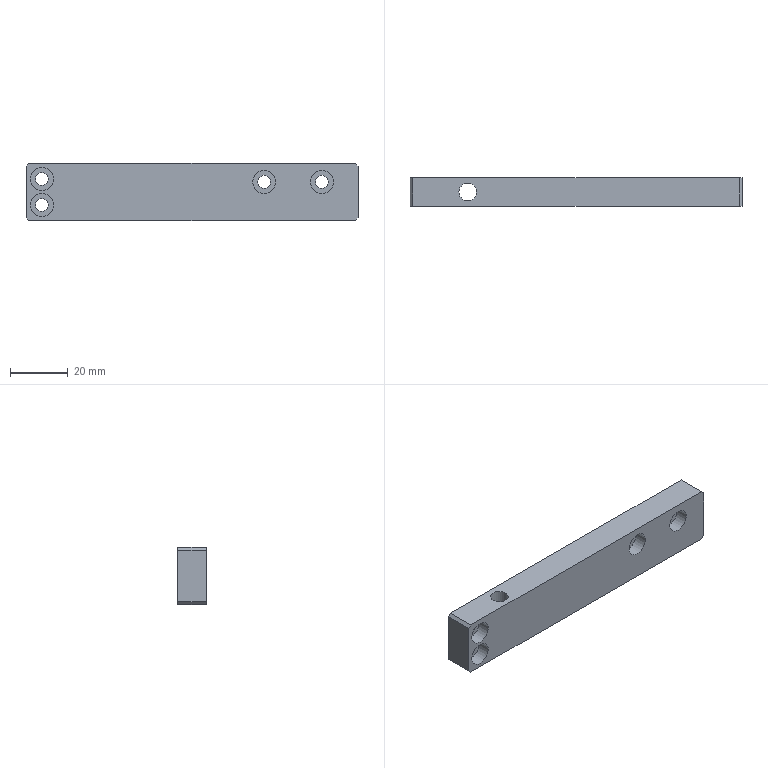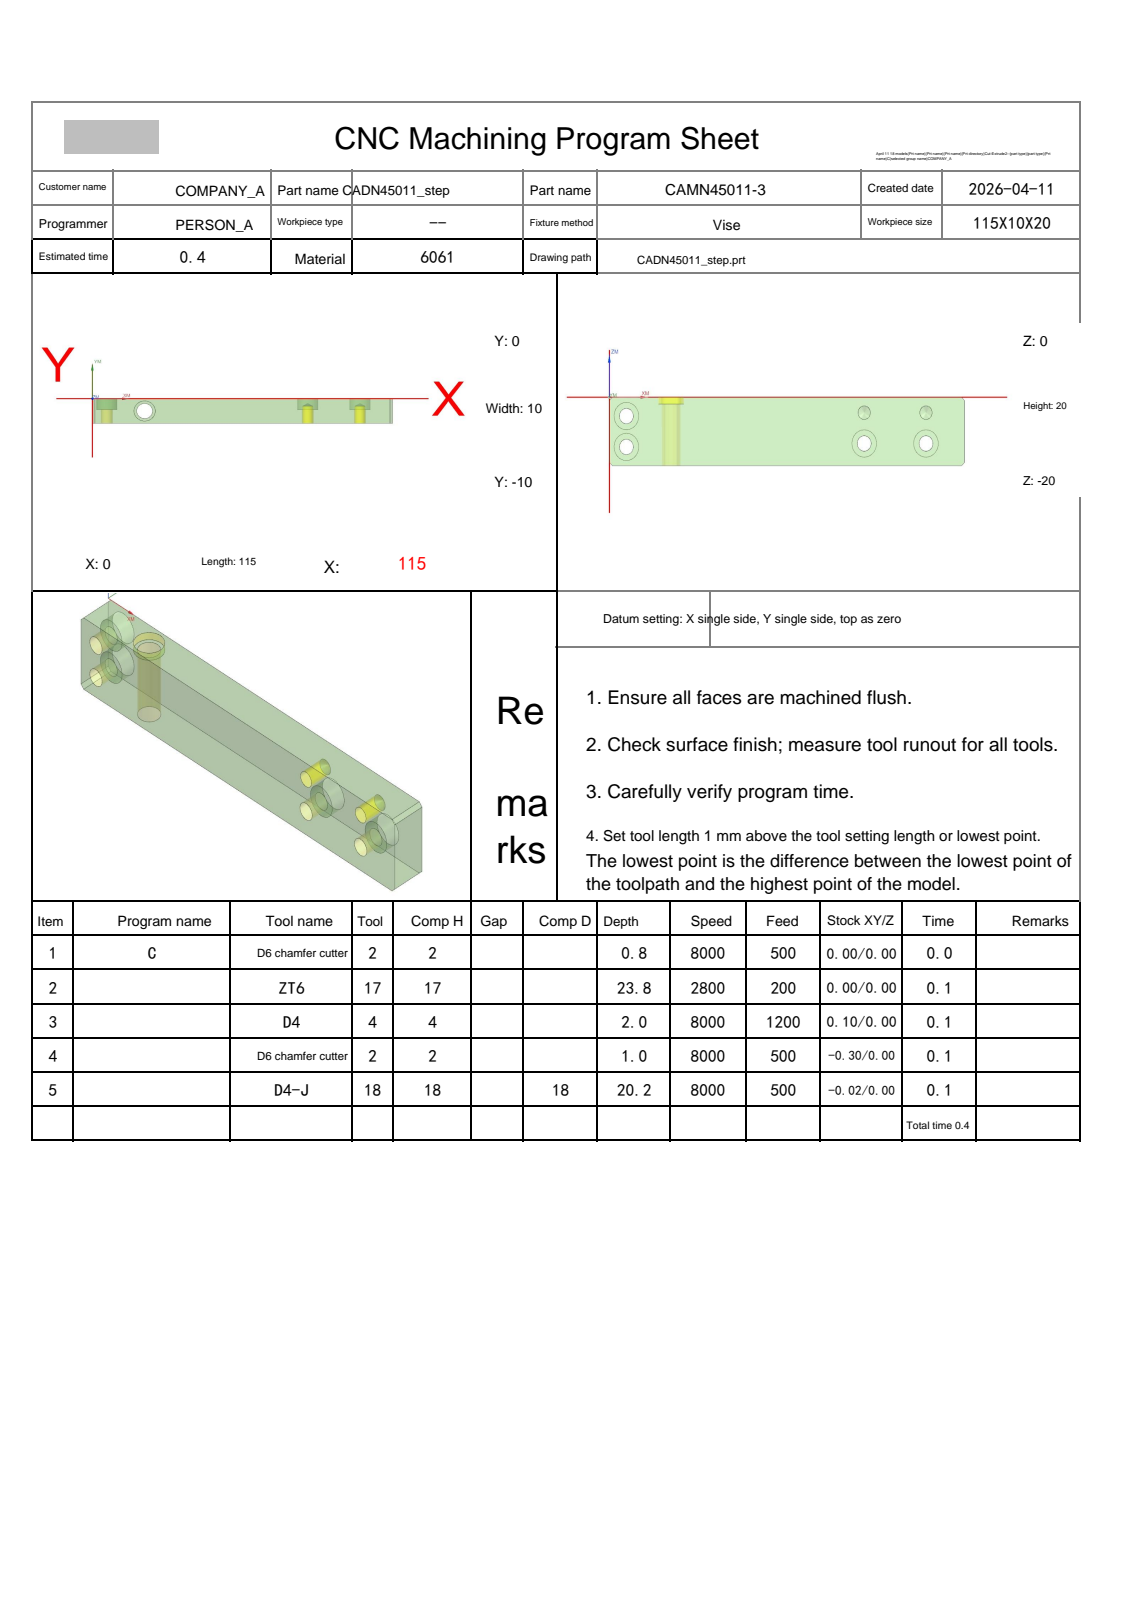NC program | NX | posted by the shop | part box 115 x 10 x 20 mm
Whole program:
%
O0001
(Machine time: 1.46 MIN)
(===Total Tool:4===)
(T2=D6 chamfer cutter   D=6.   R=0.   D-  H02 Z=-1.   )
(T17=ZT6    D=6.   DR_a=118 D-  H17 Z=-23.8 )
(T4=D4      D=4.   R=0.   D-  H04 Z=-2.   )
(T18=D4-J   D=4.   R=0.   D18 H18 Z=-20.2 )
G80 G90 G17 G49 G40
G91 G28 Z0
M01
N1 T02 M06
(D6 chamfer cutter  D=6. R=0. H=02 ce=0.00 di=0.00)
G00 G90 G54 X20. Y-5. M03 S8000
G43 H02 Z20.
M08
G98 G81 X20. Y-5. Z-.8 R1. F500.
G80
G00 Z20.
G91 G28 Z0.0
M05
M09
G91 G28 Z0.0
M01
N2 T17 M06
(ZT6 D=6. DR_a=118 H=17)
G00 G90 G54 X20. Y-5. M03 S2800
G43 H17 Z20.
M08
G98 G83 X20. Y-5. Z-23.803 R1. F200. Q2.
G80
G00 Z20.
G91 G28 Z0.0
M05
M09
G91 G28 Z0.0
M01
N3 T04 M06
(D4  D=4. R=0. H=04 ce=0.10 di=0.00)
G00 G90 G54 X20. Y-5. M03 S8000
G43 H04 Z20.
M08
Z.5
G03 X21. Y-6. I1. J0.0 F1200.
X22. Y-5. I0.0 J1.
X22. Y-5. Z.2 I-2. J0.0
X22. Y-5. Z-.1 I-2. J0.0
X22. Y-5. Z-.4 I-2. J0.0
X22. Y-5. Z-.7 I-2. J0.0
X22. Y-5. Z-1. I-2. J0.0
X22. Y-5. Z-1.3 I-2. J0.0
X22. Y-5. Z-1.6 I-2. J0.0
X22. Y-5. Z-1.9 I-2. J0.0
X19. Y-3.268 Z-2. I-2. J0.0
X18. Y-5. I1. J-1.732
X20. Y-7. I2. J0.0
X22. Y-5. I0.0 J2.
X20. Y-3. I-2. J0.0
X19. Y-3.268 I0.0 J-2.
X18.5 Y-4.134 I.5 J-.866
X19.5 Y-5.134 I1. J0.0
X20. Y-5. I0.0 J1.
G00 Z20.
G91 G28 Z0.0
M05
M09
G91 G28 Z0.0
M01
N4 T02 M06
(D6 chamfer cutter  D=6. R=0. H=02 ce=-0.30 di=0.00)
G00 G90 G54 X23.233 Y-3.949 M03 S8000
G43 H02 Z20.
M08
Z2.5
G01 X23.116 Y-3.631 Z2.377 F500.
X22.932 Y-3.273 Z2.23
X22.708 Y-2.939 Z2.084
X22.446 Y-2.634 Z1.937
X22.15 Y-2.362 Z1.791
X21.824 Y-2.127 Z1.645
X21.576 Y-1.984 Z1.541
X21.209 Y-1.819 Z1.394
X20.826 Y-1.699 Z1.248
X20.43 Y-1.624 Z1.101
X20.029 Y-1.597 Z.955
X19.627 Y-1.617 Z.809
X19.231 Y-1.685 Z.662
X18.845 Y-1.799 Z.516
X18.476 Y-1.958 Z.37
X18.127 Y-2.159 Z.223
X17.805 Y-2.399 Z.077
X17.514 Y-2.677 Z-.07
X17.257 Y-2.986 Z-.216
X17.038 Y-3.324 Z-.362
X16.861 Y-3.685 Z-.509
X16.728 Y-4.064 Z-.655
X16.641 Y-4.457 Z-.802
X16.6 Y-4.857 Z-.948
Y-5. Z-1.
G03 X20. Y-8.4 I3.4 J0.0
X23.4 Y-5. I0.0 J3.4
X20. Y-1.6 I-3.4 J0.0
X16.6 Y-5. I0.0 J-3.4
X16.637 Y-5.498 I3.4 J0.0
G01 Z1.5
G00 Z20.
G91 G28 Z0.0
M05
M09
G91 G28 Z0.0
M01
N5 T18 M06
(D4-J  D=4. R=0. H=18 ce=-0.02 di=0.00)
G00 G90 G54 X19.2 Y-5.85 M03 S8000
G43 H18 Z10.
M08
Z-1.
G01 Z-2. F500.
G41 D18
Y-6.32
G03 X20. Y-7.12 I.8 J0.0
X22.12 Y-5. I0.0 J2.12
X20. Y-2.88 I-2.12 J0.0
X17.88 Y-5. I0.0 J-2.12
X20. Y-7.12 I2.12 J0.0
X20.398 Y-7.082 I0.0 J2.12
X21.048 Y-6.297 I-.15 J.786
G01 X21.033 Y-6.147
X20.983 Y-5.881
G40 X20.945 Y-5.685
Z-1.
G00 Z10.
G00 G90 X20.37 Y-4.71 M03 S8000
Z10.
Z-5.05
G01 Z-6.55 F500.
G41 D18
X20.6 Y-4.53
G03 X20. Y-3.93 I-.6 J0.0
X18.93 Y-5. I0.0 J-1.07
X20. Y-6.07 I1.07 J0.0
X21.07 Y-5. I0.0 J1.07
X20. Y-3.93 I-1.07 J0.0
X19.609 Y-4.004 I0.0 J-1.07
X19.228 Y-4.562 I.219 J-.559
X19.27 Y-4.782 I.6 J0.0
G01 G40 X19.55 Y-4.865
Z-5.05
G00 X20.37 Y-4.71
Z-9.6
G01 Z-11.1
G41 D18
X20.6 Y-4.53
G03 X20. Y-3.93 I-.6 J0.0
X18.93 Y-5. I0.0 J-1.07
X20. Y-6.07 I1.07 J0.0
X21.07 Y-5. I0.0 J1.07
X20. Y-3.93 I-1.07 J0.0
X19.609 Y-4.004 I0.0 J-1.07
X19.228 Y-4.562 I.219 J-.559
X19.27 Y-4.782 I.6 J0.0
G01 G40 X19.55 Y-4.865
Z-9.6
G00 X20.37 Y-4.71
Z-14.15
G01 Z-15.65
G41 D18
X20.6 Y-4.53
G03 X20. Y-3.93 I-.6 J0.0
X18.93 Y-5. I0.0 J-1.07
X20. Y-6.07 I1.07 J0.0
X21.07 Y-5. I0.0 J1.07
X20. Y-3.93 I-1.07 J0.0
X19.609 Y-4.004 I0.0 J-1.07
X19.228 Y-4.562 I.219 J-.559
X19.27 Y-4.782 I.6 J0.0
G01 G40 X19.55 Y-4.865
Z-14.15
G00 X20.37 Y-4.71
Z-18.7
G01 Z-20.2
G41 D18
X20.6 Y-4.53
G03 X20. Y-3.93 I-.6 J0.0
X18.93 Y-5. I0.0 J-1.07
X20. Y-6.07 I1.07 J0.0
X21.07 Y-5. I0.0 J1.07
X20. Y-3.93 I-1.07 J0.0
X19.609 Y-4.004 I0.0 J-1.07
X19.228 Y-4.562 I.219 J-.559
X19.27 Y-4.782 I.6 J0.0
G01 G40 X19.55 Y-4.865
Z-18.7
G00 Z10.
M05
M09
G91 G28 Z0.0
G91 G28 Y0.0
M30
%